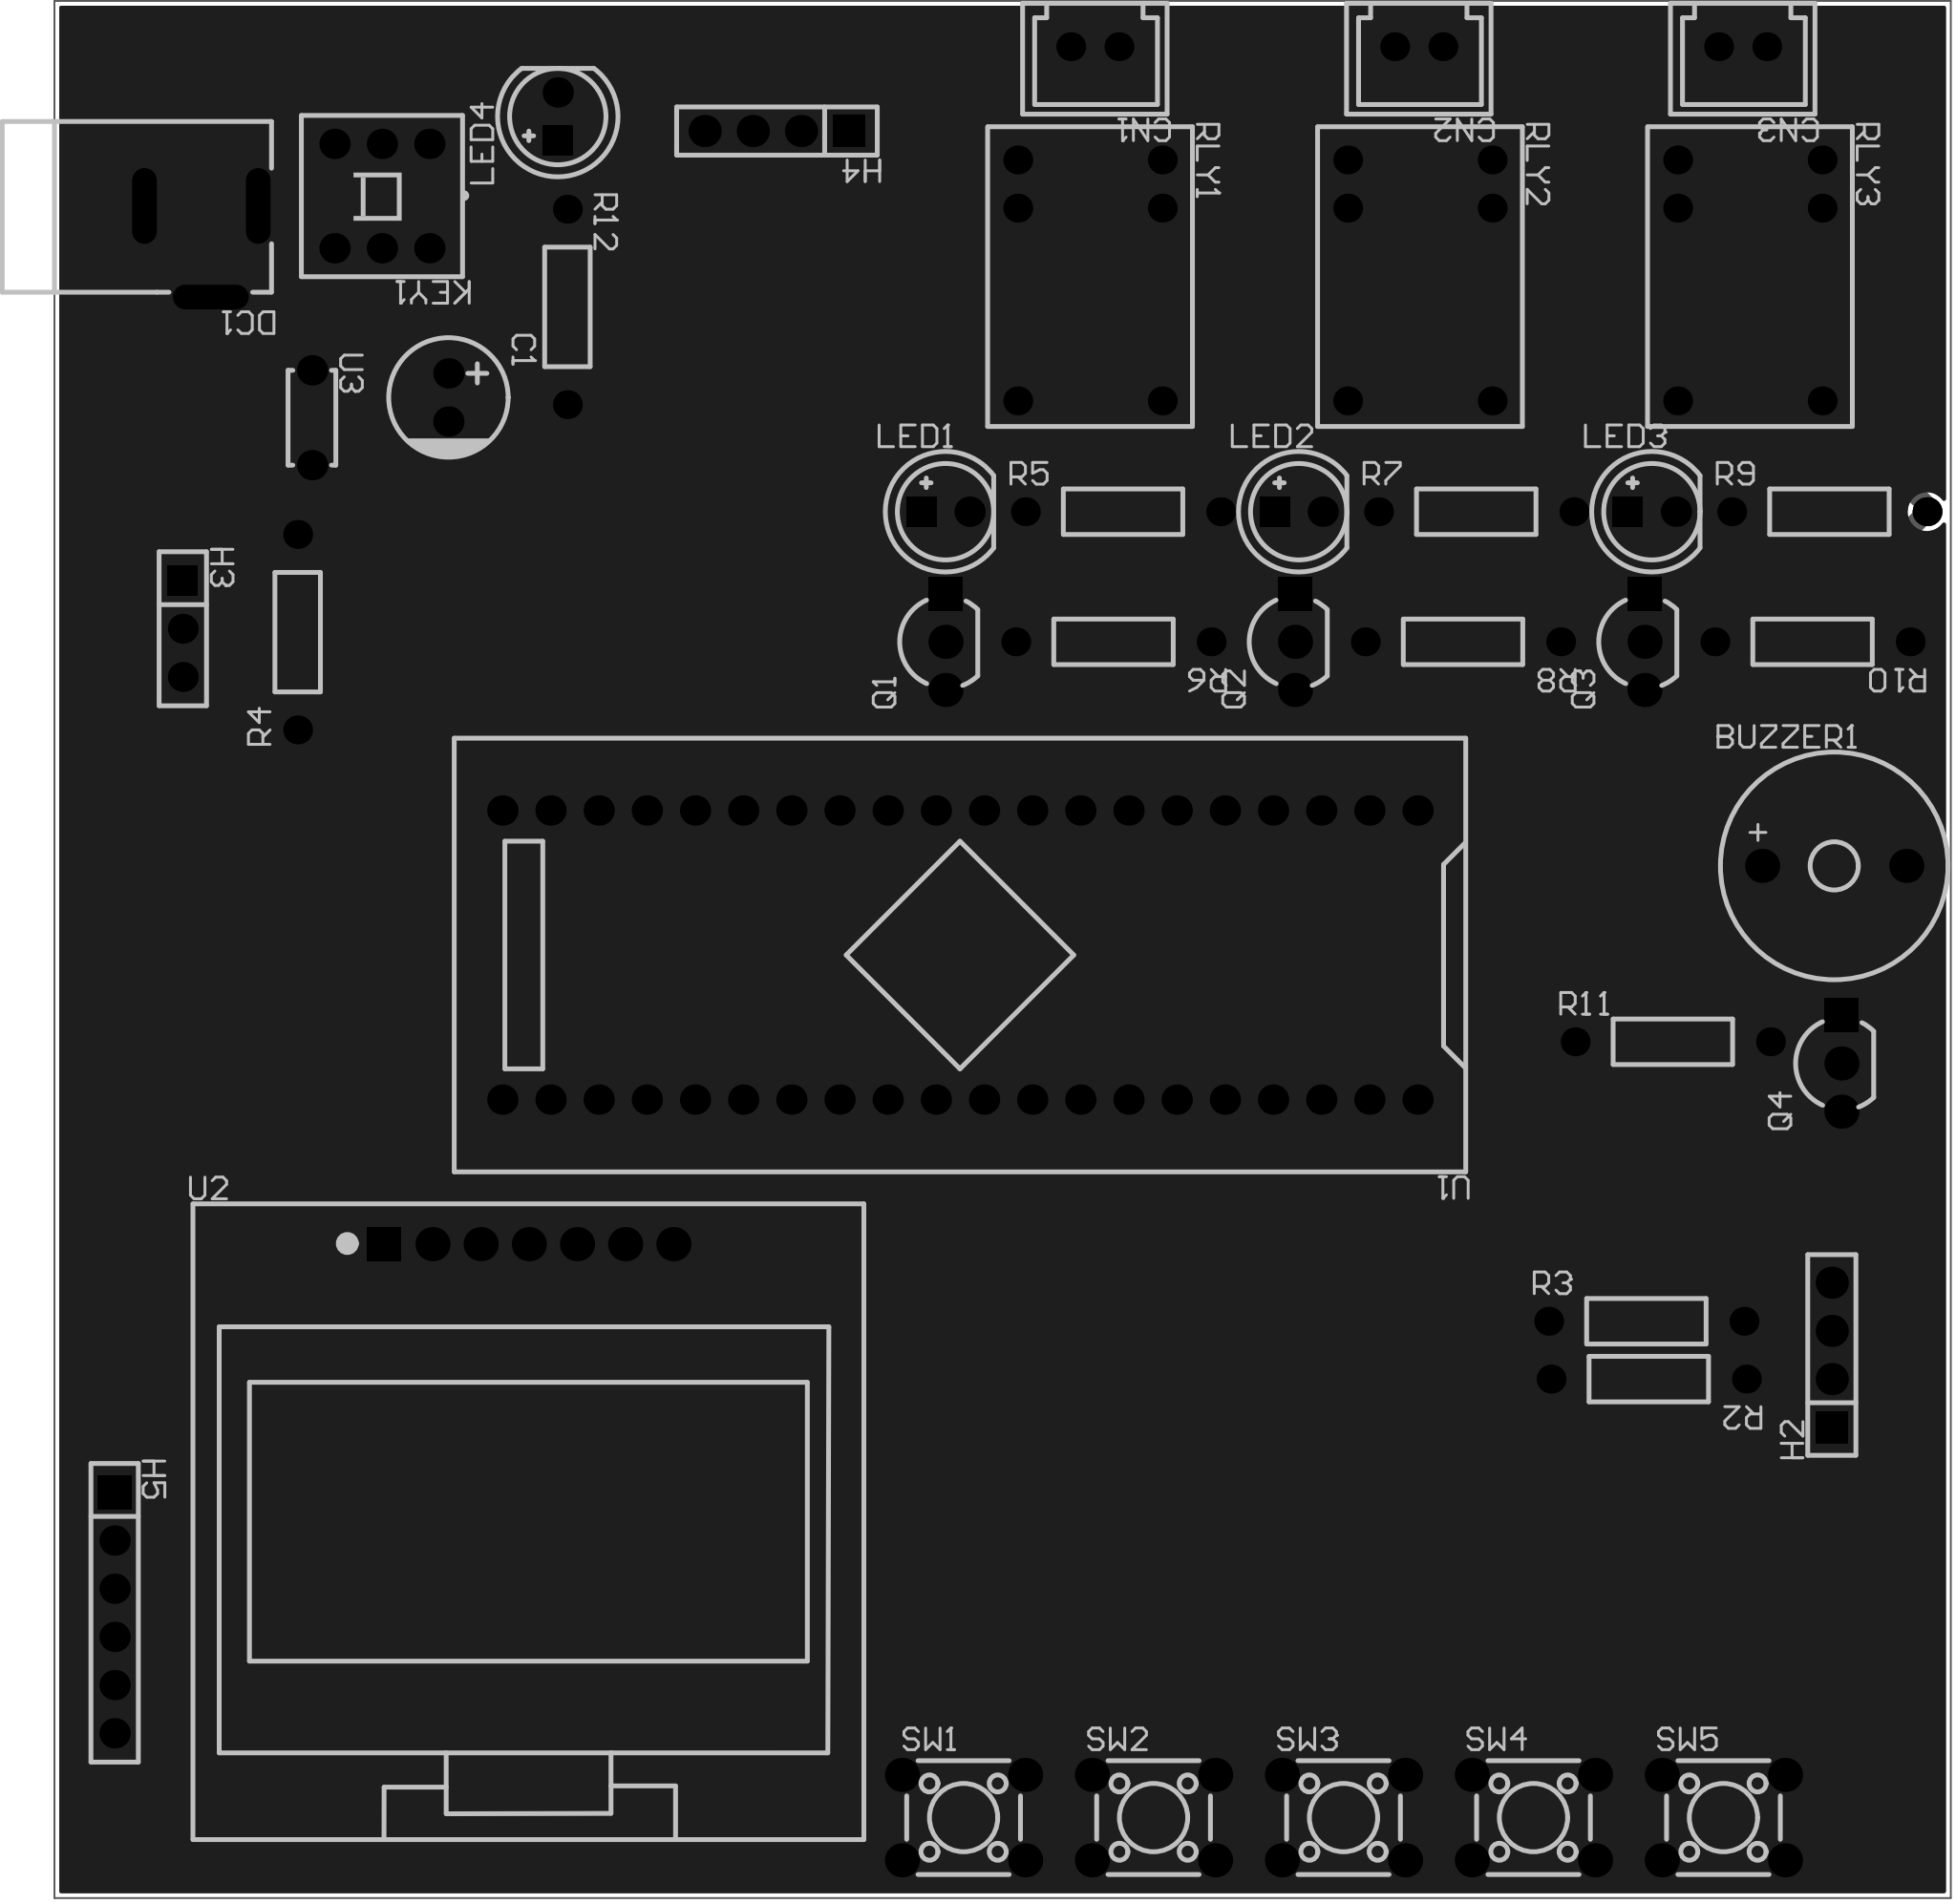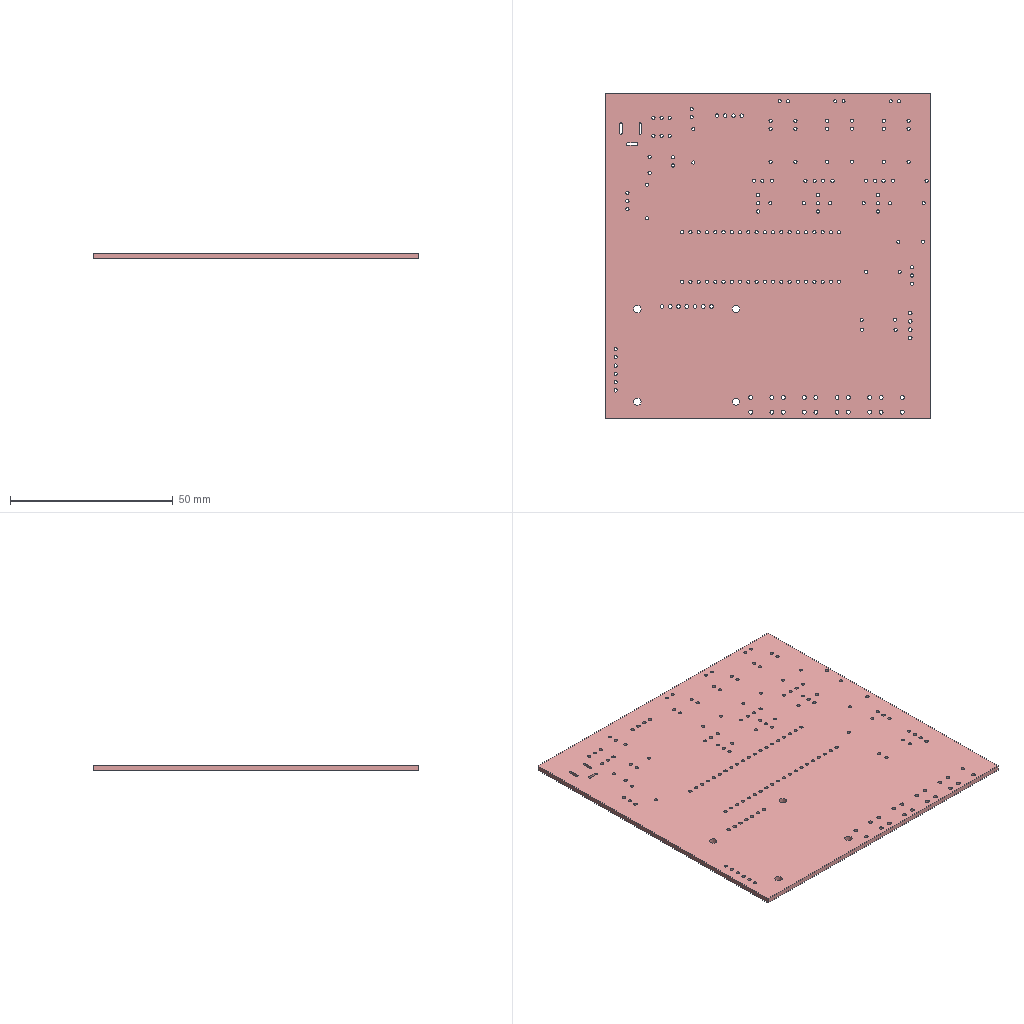Circuit board layout | Altium Designer | box 100 x 100 x 1.6 mm
Layer stack:
# Altium Designer layer stack of  (unit mm; dielectric type: 0 none, 1 core, 2 prepreg, 3 surface material)
index,name,kind,layer,copper_thickness_mm,dielectric_type,dielectric_thickness_mm,dielectric_material,dielectric_constant
0,Top Paste Mask Layer,other,,,,,,
1,Top Silkscreen Layer,other,,,,,,
2,Top Solder Mask Layer,dielectric,,,3,0.01,,3.3
3,Top Layer,copper,Top Layer,0.035,,,,
4,Dielectric1,dielectric,,,3,1.51,FR4,4.5
5,Bottom Layer,copper,Bottom Layer,0.035,,,,
6,Bottom Solder Mask Layer,dielectric,,,3,0.01,,3.3
7,Bottom Silkscreen Layer,other,,,,,,
8,Bottom Paste Mask Layer,other,,,,,,
# drill layer pairs: low layer,high layer
drill_pair,Top Layer,Bottom Layer
Part placement:
Designator,Comment,Layer,Footprint,Center-X(mm),Center-Y(mm),Rotation
BUZZER1,buzzer-12X9,TopLayer,BUZ-TH_BD12.0-P7.60-D0.6-FD,184.785,139.573,0
C1,220uF,TopLayer,CAP-TH_BD6.3-P2.50-D1.0-FD,111.709,164.265,270
CN1,2P PH2.54,TopLayer,CONN-TH_2P-P2.54_HDR2,145.796,182.753,180
CN2,2P PH2.54,TopLayer,CONN-TH_2P-P2.54_HDR2,162.877,182.753,180
CN3,2P PH2.54,TopLayer,CONN-TH_2P-P2.54_HDR2,179.959,182.753,180
DC1,,TopLayer,DC-2.0,98.679,171.958,180
H2,,TopLayer,HDR-TH_4P-P2.54-V-F,184.658,113.792,90
H3,,TopLayer,HDR-TH_3P-P2.54-V-F,97.702,152.073,270
H4,,TopLayer,HDR-TH_4P-P2.54-V-F,129.032,178.308,180
H5,,TopLayer,HDR-TH_6P-P2.54-V-F,94.107,100.203,270
KEY1,Non-latching switch 8.5×8.5 silent,TopLayer,SW-TH_6P-L8.5-W8.5-P2.54,108.204,174.879,180
LED1,,TopLayer,LED-TH_5mm,137.922,158.242,0
LED2,,TopLayer,LED-TH_5mm,156.546,158.242,0
LED3,,TopLayer,LED-TH_5mm,175.169,158.242,0
LED4,,TopLayer,LED-TH_5mm,117.475,179.07,90
Q1,9013,TopLayer,TO-92-3_L4.8-W3.7-P2.54-R,137.922,151.384,90
Q2,9013,TopLayer,TO-92-3_L4.8-W3.7-P2.54-R,156.353,151.384,90
Q3,9013,TopLayer,TO-92-3_L4.8-W3.7-P2.54-R,174.785,151.384,90
Q4,9013,TopLayer,TO-92-3_L4.8-W3.7-P2.54-R,185.166,129.159,90
R2,10kΩ,TopLayer,Res_1/4W,175.006,112.522,180
R3,5kΩ,TopLayer,Res_1/4W,174.879,115.57,0
R4,5kΩ,TopLayer,Res_1/4W,103.759,151.892,90
R5,5kΩ,TopLayer,Res_1/4W,147.284,158.242,0
R6,5kΩ,TopLayer,Res_1/4W,146.779,151.384,180
R7,5kΩ,TopLayer,Res_1/4W,165.907,158.242,0
R8,5kΩ,TopLayer,Res_1/4W,165.211,151.384,180
R9,5kΩ,TopLayer,Res_1/4W,184.531,158.242,0
R10,5kΩ,TopLayer,Res_1/4W,183.642,151.384,180
R11,5kΩ,TopLayer,Res_1/4W,176.276,130.302,0
R12,5kΩ,TopLayer,Res_1/4W,117.983,169.037,270
RLY1,SRS-05VDC-SL-C,TopLayer,RELAY-TH_SRS-05VDC-SL-C,145.542,170.434,270
RLY2,SRS-05VDC-SL-C,TopLayer,RELAY-TH_SRS-05VDC-SL-C,162.941,170.434,270
RLY3,SRS-05VDC-SL-C,TopLayer,RELAY-TH_SRS-05VDC-SL-C,180.34,170.434,270
SW1,,TopLayer,SW-TH_4P-L6.0-W6.0-P4.50-LS6.5,138.874,89.408,180
SW2,,TopLayer,SW-TH_4P-L6.0-W6.0-P4.50-LS6.5,148.892,89.408,180
SW3,,TopLayer,SW-TH_4P-L6.0-W6.0-P4.50-LS6.5,158.909,89.408,180
SW4,,TopLayer,SW-TH_4P-L6.0-W6.0-P4.50-LS6.5,168.926,89.408,180
SW5,,TopLayer,SW-TH_4P-L6.0-W6.0-P4.50-LS6.5,178.943,89.408,180
U1,STM32F103C8T6-Card,TopLayer,CONN-TH_L53.3-W22.9_STM32F103C8T6-CARD,138.684,134.874,180
U2,1.30OLED_7P,TopLayer,LCD-TH_7P-P2.54_1.30OLED_7P,115.951,119.634,0
U3,100nF,TopLayer,CAP-TH_L5.0-W2.5-P5.00-D1.0,104.521,163.195,270
Pad and via stacks:
# Altium Designer via and pad stacks of  (unit mm). Each distinct definition once, with the count of objects using it.
# via: kind,start_layer,end_layer,hole_mm,diameter_mm,mode(0 simple;1 top-mid-bottom;2 full stack),diameter_per_layer,count,example_net
# pad: kind,layer,hole_mm,hole_type(0 round;1 square;2 slot),plating,top_size,top_shape(1 round;2 rect;3 octagon;9 rounded rect),mid_size,bottom_size,mode,footprint,size_per_layer,count,example
pad,Multi-Layer,1,0,plated,1.8x1.8,1,1.8x1.8,1.8x1.8,0,BUZ-TH_BD12.0-P7.60-D0.6-FD,,2,BUZZER1.2
pad,Multi-Layer,1,0,plated,1.6x1.6,1,1.6x1.6,1.6x1.6,0,CAP-TH_BD6.3-P2.50-D1.0-FD,,2,C1.1
pad,Multi-Layer,0.9144,0,plated,1.524x1.524,1,1.524x1.524,1.524x1.524,0,CONN-TH_2P-P2.54_HDR2,,6,CN1.1
pad,Multi-Layer,0.8001,2,plated,4x1.3,1,4x1.3,4x1.3,0,DC-2.0,,3,DC1.2
pad,Multi-Layer,1.1,0,plated,1.7x1.7,2,1.7x1.7,1.7x1.7,0,HDR-TH_4P-P2.54-V-F,,2,H2.1
pad,Multi-Layer,1.1,0,plated,1.7x1.7,1,1.7x1.7,1.7x1.7,0,HDR-TH_4P-P2.54-V-F,,6,H2.2
pad,Multi-Layer,1.02,0,plated,1.575x1.575,1,1.575x1.575,1.575x1.575,0,HDR-TH_3P-P2.54-V-F,,2,H3.3
pad,Multi-Layer,1.02,0,plated,1.575x1.575,2,1.575x1.575,1.575x1.575,0,HDR-TH_3P-P2.54-V-F,,1,H3.1
pad,Multi-Layer,1.02,0,plated,1.6x1.6,1,1.6x1.6,1.6x1.6,0,HDR-TH_6P-P2.54-V-F,,5,H5.6
pad,Multi-Layer,1.02,0,plated,1.8x1.8,2,1.8x1.8,1.8x1.8,0,HDR-TH_6P-P2.54-V-F,,1,H5.1
pad,Multi-Layer,1,0,plated,1.6x1.6,1,1.6x1.6,1.6x1.6,0,SW-TH_6P-L8.5-W8.5-P2.54,,6,KEY1.4
pad,Multi-Layer,1,0,plated,1.6x1.6,2,1.6x1.6,1.6x1.6,0,LED-TH_5mm,,4,LED1.1
pad,Multi-Layer,1,0,plated,1.6x1.6,1,1.6x1.6,1.6x1.6,0,LED-TH_5mm,,4,LED1.2
pad,Multi-Layer,1,0,plated,1.8x1.8,2,1.8x1.8,1.8x1.8,0,TO-92-3_L4.8-W3.7-P2.54-R,,4,Q1.1
pad,Multi-Layer,1,0,plated,1.8x1.8,1,1.8x1.8,1.8x1.8,0,TO-92-3_L4.8-W3.7-P2.54-R,,8,Q1.2
pad,Multi-Layer,1,0,plated,1.524x1.524,1,1.524x1.524,1.524x1.524,0,Res_1/4W,,22,R2.1
pad,Multi-Layer,1,0,plated,1.524x1.524,1,1.524x1.524,1.524x1.524,0,RELAY-TH_SRS-05VDC-SL-C,,18,RLY1.1
pad,Multi-Layer,1.2,0,plated,1.8x1.8,1,1.8x1.8,1.8x1.8,0,SW-TH_4P-L6.0-W6.0-P4.50-LS6.5,,20,SW1.1
pad,Multi-Layer,1,0,plated,1.6x1.6,1,1.6x1.6,1.6x1.6,0,CONN-TH_L53.3-W22.9_STM32F103C8T6-CARD,,40,U1.1
pad,Multi-Layer,1.1,0,plated,1.802x1.802,1,1.802x1.802,1.802x1.802,0,LCD-TH_7P-P2.54_1.30OLED_7P,,1,U2.7
pad,Multi-Layer,1.1,0,plated,1.802x1.802,1,1.802x1.802,1.802x1.802,0,LCD-TH_7P-P2.54_1.30OLED_7P,,5,U2.6
pad,Multi-Layer,1.1,0,plated,1.802x1.802,2,1.802x1.802,1.802x1.802,0,LCD-TH_7P-P2.54_1.30OLED_7P,,1,U2.1
pad,Multi-Layer,1,0,plated,1.6x1.6,1,1.6x1.6,1.6x1.6,0,CAP-TH_L5.0-W2.5-P5.00-D1.0,,2,U3.1
Copper pours:
name,layer,net,type(0 solid;1 hatched;2 none)
Top Layer-GND,Top Layer,GND,0
Bottom Layer-GND,Bottom Layer,GND,0